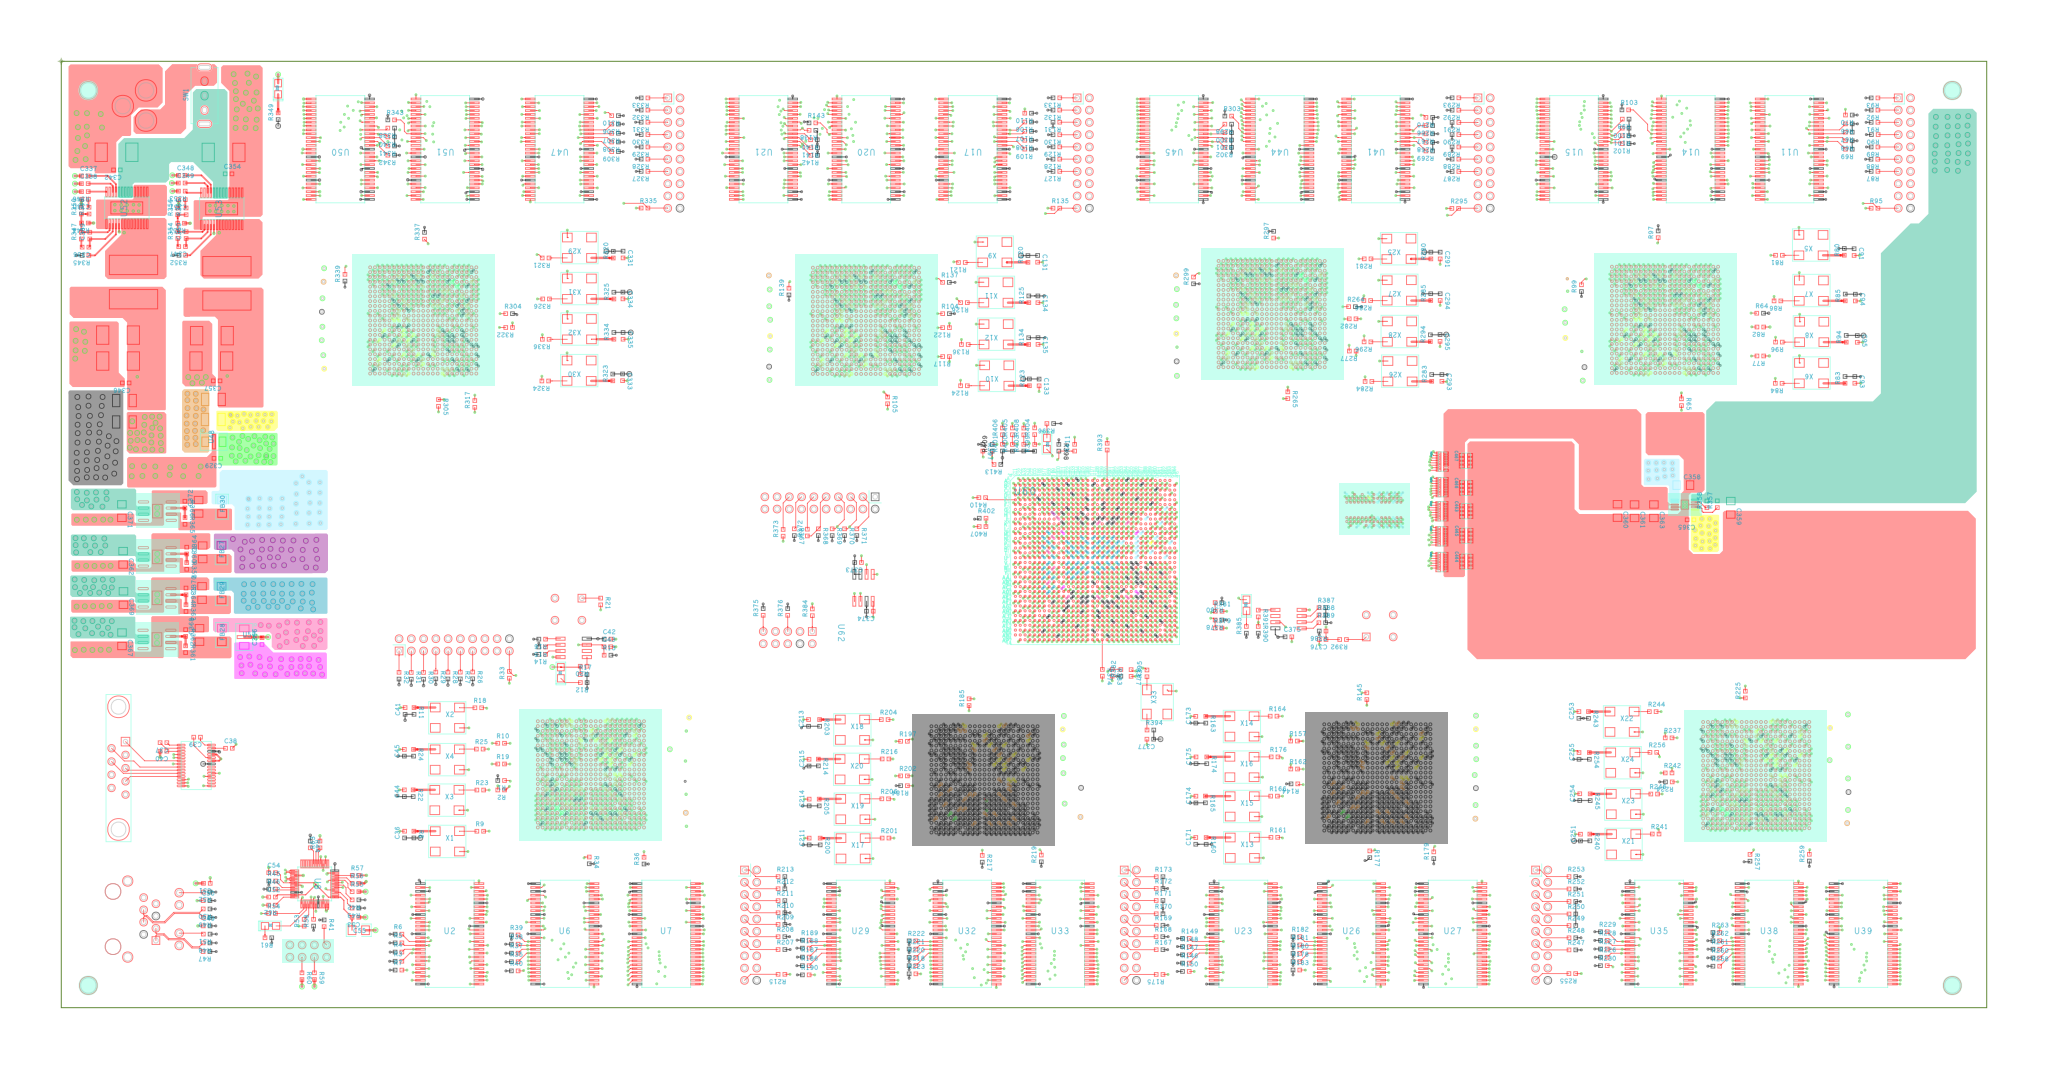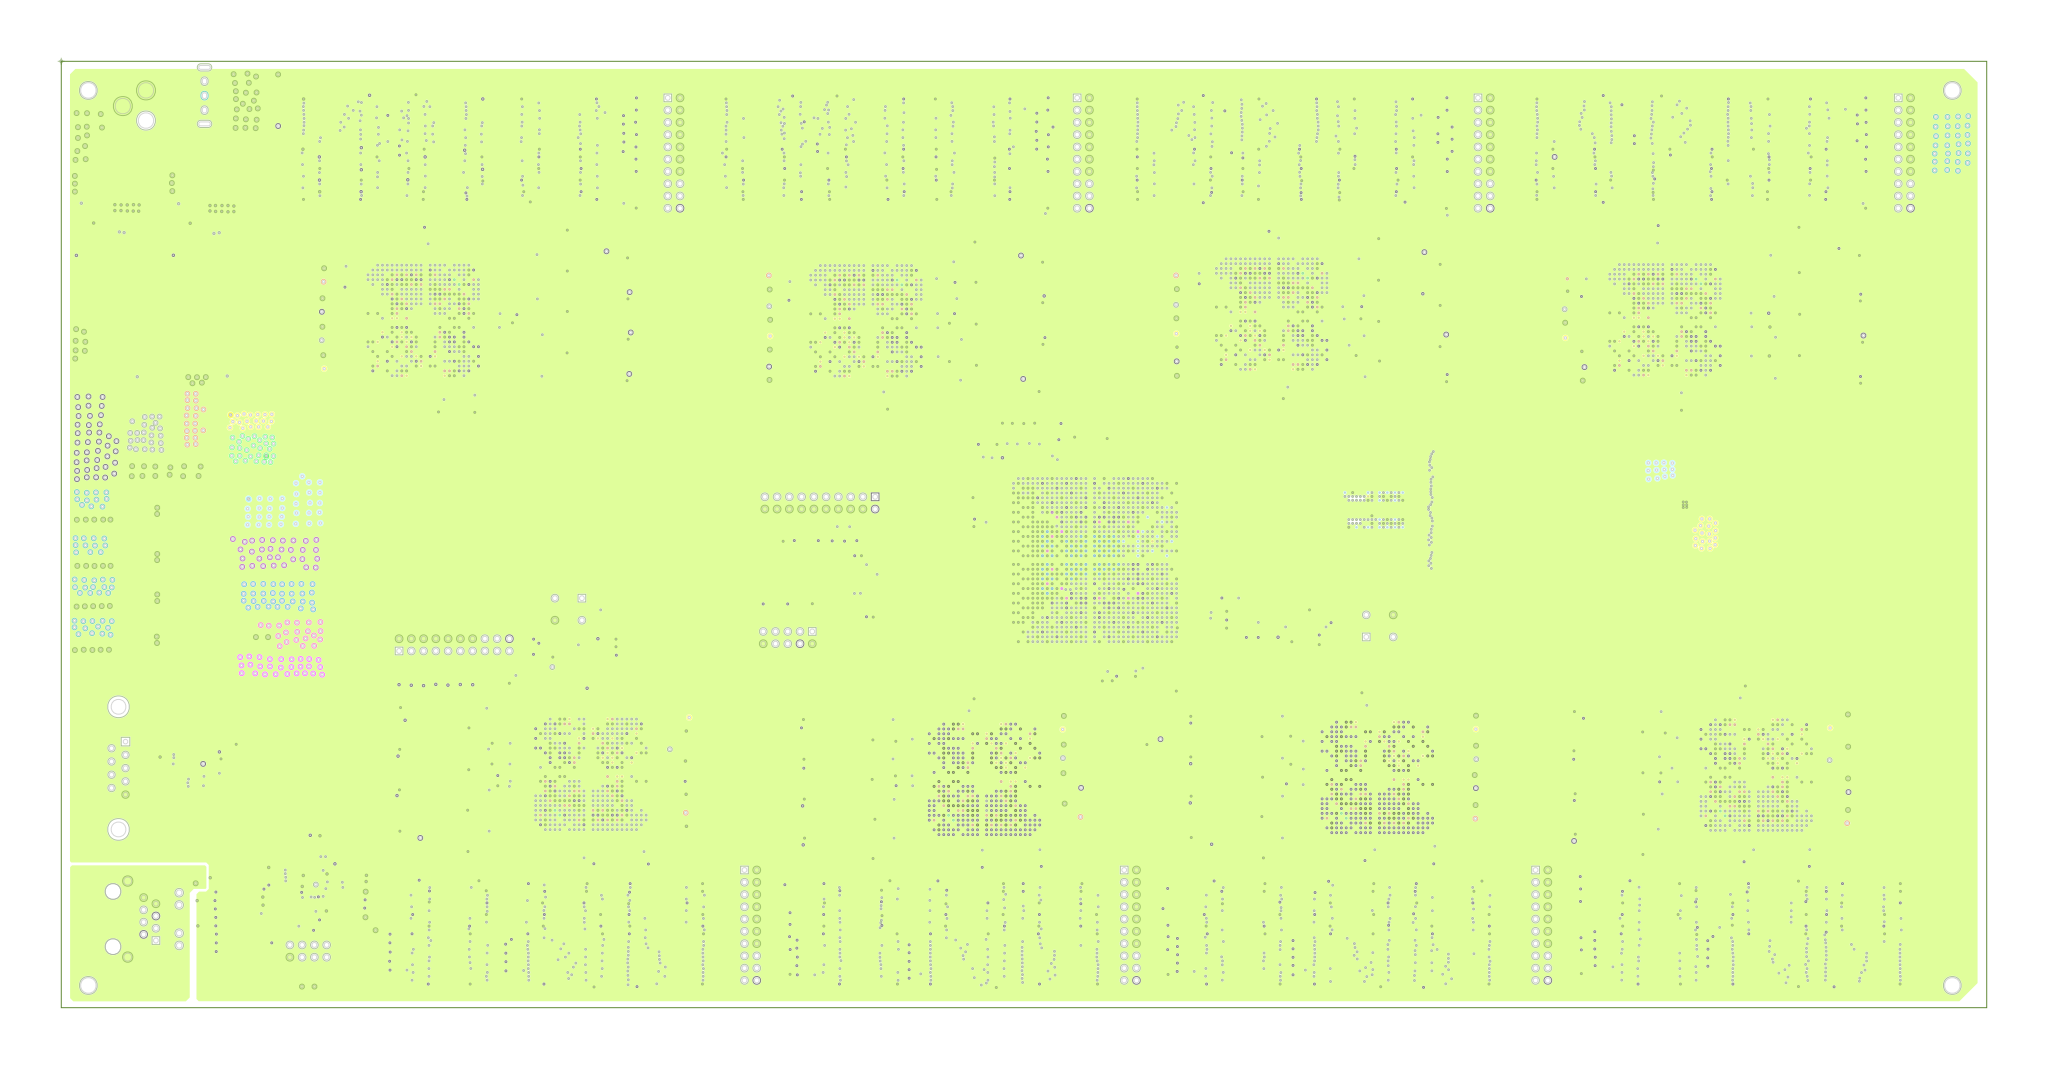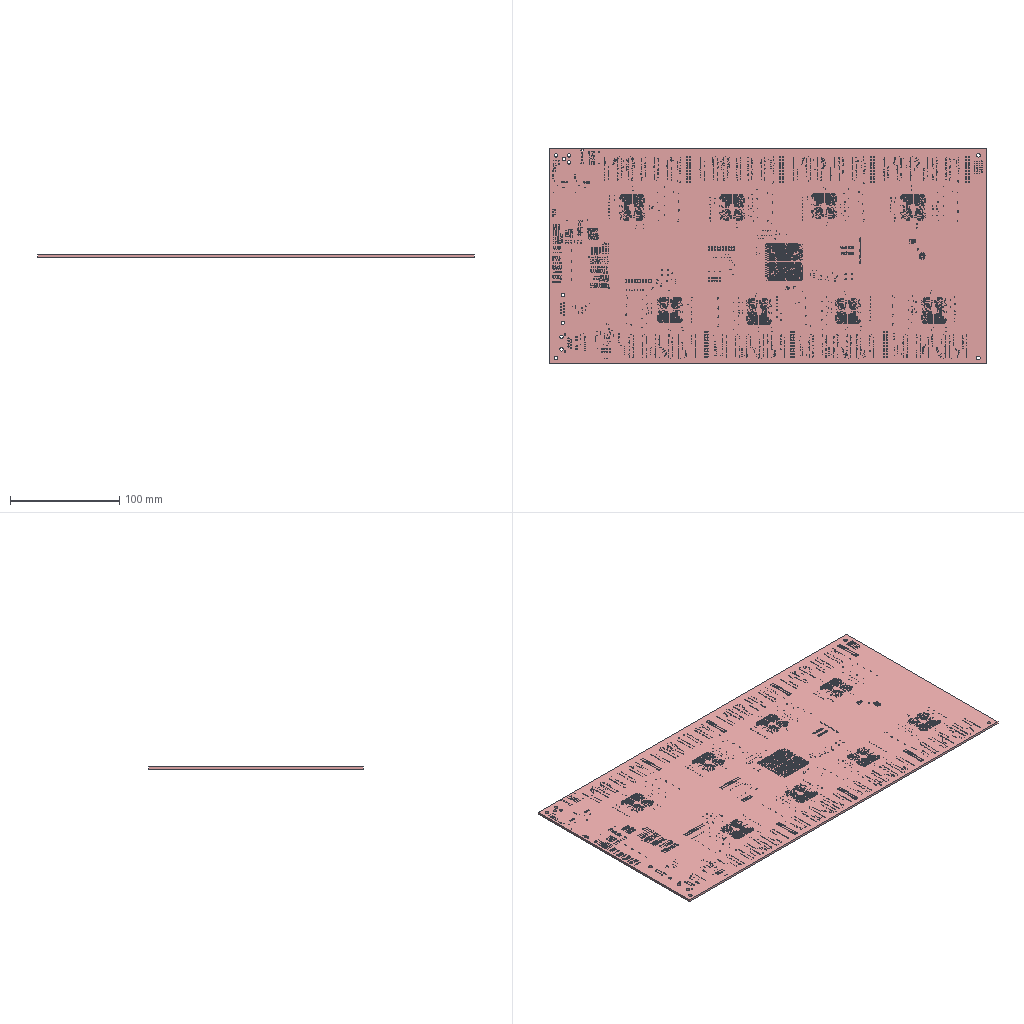Circuit board layout | Cadence Allegro | box 399 x 196 x 2.1 mm
Layer stack:
# Cadence Allegro layer stack of  (unit mm; from the constraint file cross-section; dielectric type: 0 not recorded (Allegro does not mark core vs prepreg), 3 surface material)
index,name,kind,layer,copper_thickness_mm,dielectric_type,dielectric_thickness_mm,dielectric_material,dielectric_constant
0,Top Surface,other,,,,,,
1,TOP,copper,TOP,0.0305,,,,
2,Dielectric1,dielectric,,,0,0.2032,FR-4,4.5
3,GND2,copper,GND2,0.0305,,,,
4,Dielectric2,dielectric,,,0,0.2032,FR-4,4.5
5,SIG3,copper,SIG3,0.0305,,,,
6,Dielectric3,dielectric,,,0,0.2032,FR-4,4.5
7,SIG4,copper,SIG4,0.0305,,,,
8,Dielectric4,dielectric,,,0,0.2032,FR-4,4.5
9,POWER5,copper,POWER5,0.0305,,,,
10,Dielectric5,dielectric,,,0,0.2032,FR-4,4.5
11,SIG6,copper,SIG6,0.0305,,,,
12,Dielectric6,dielectric,,,0,0.2032,FR-4,4.5
13,GND7,copper,GND7,0.0305,,,,
14,Dielectric7,dielectric,,,0,0.2032,FR-4,4.5
15,SIG8,copper,SIG8,0.0305,,,,
16,Dielectric8,dielectric,,,0,0.2032,FR-4,4.5
17,POWER9,copper,POWER9,0.0305,,,,
18,Dielectric9,dielectric,,,0,0.2032,FR-4,4.5
19,BOTTOM,copper,BOTTOM,0.0305,,,,
20,Bottom Surface,other,,,,,,
# drill layer pairs: low layer,high layer
drill_pair,TOP,BOTTOM
Part placement, first 571 of 1006 lines:
REFDES,COMP_VALUE,SYM_NAME,SYM_X,SYM_Y,SYM_ROTATE,SYM_MIRROR
C1,10uF,C3216,5033.571,-5866.500,90.000,YES
C2,0.1uF,C0402,3908.307,-6248.500,180.000,YES
C3,0.1uF,C0402,4125.307,-5754.500,0.000,YES
C4,0.1uF,C0402,4606.500,-5965.622,270.000,YES
C5,0.1uF,C0402,4302.000,-6161.000,90.000,YES
C6,0.1uF,C0402,4765.000,-5437.000,90.000,YES
C7,0.1uF,C0402,4417.984,-5762.138,315.000,YES
C8,0.1uF,C0402,4702.713,-5683.752,225.000,YES
C9,0.1uF,C0402,3913.441,-5652.004,135.000,YES
C10,0.1uF,C0402,3901.358,-5417.583,135.000,YES
C11,0.1uF,C0402,3905.429,-5551.500,180.000,YES
C12,0.1uF,C0402,4415.220,-5444.098,225.000,YES
C13,0.1uF,C0402,4646.776,-5509.992,90.000,YES
C14,0.1uF,C0402,4006.571,-5817.500,270.000,YES
C15,10uF,C3216,5032.307,-6127.500,90.000,YES
C16,0.1uF,C0402,4058.996,-5880.287,225.000,YES
C17,0.1uF,C0402,4724.693,-5514.500,90.000,YES
C18,0.1uF,C0402,4293.307,-5562.500,180.000,YES
C19,0.1uF,C0402,4105.307,-5439.500,0.000,YES
C20,0.1uF,C0402,4301.500,-5475.307,270.000,YES
C21,0.1uF,C0402,4221.264,-5740.500,90.000,YES
C22,0.1uF,C0402,4263.500,-5901.736,270.000,YES
C23,0.1uF,C0402,4475.736,-5868.500,180.000,YES
C24,0.1uF,C0402,4302.622,-6069.500,270.000,YES
C25,0.1uF,C0402,4547.343,-6157.555,135.000,YES
C26,0.1uF,C0402,4696.327,-5817.551,135.000,YES
C27,0.1uF,C0402,4809.378,-5617.500,90.000,YES
C28,10uF,C3216,5034.307,-5609.500,90.000,YES
C29,0.1uF,C0402,4120.500,-5320.693,0.000,YES
C30,0.1uF,C0402,4193.307,-5490.500,270.000,YES
C31,0.1uF,C0402,4519.736,-5795.500,0.000,YES
C32,0.1uF,C0402,4611.953,-5605.512,225.000,YES
C33,10uF,C3216,5036.500,-5350.622,90.000,YES
C34,0.1uF,C0402,7198.000,-750.000,270.000,YES
C35,104,0603,1227.000,-5668.000,90.000,YES
C36,0.1uF,0603,2801.000,-6305.000,90.000,NO
C37,104,0603,833.622,-5555.500,180.000,NO
C38,104,0603,1367.500,-5601.378,0.000,NO
C39,104,0603,1108.000,-5511.000,180.000,NO
C40,104,0603,833.622,-5625.500,180.000,NO
C41,0.1uF,0603,2805.000,-5297.000,90.000,NO
C42,0.1uF,0603,4456.693,-4711.500,0.000,NO
C43,0.1uF,0603,4454.693,-4773.500,0.000,NO
C44,0.1uF,0603,2799.000,-5968.000,90.000,NO
C45,0.1uF,0603,2799.000,-5638.000,90.000,NO
C46,0.1uF,0603,2232.500,-6606.693,270.000,YES
C47,0.1uF,0603,1906.500,-6744.693,90.000,YES
C48,0.1uF,0603,2125.500,-6870.693,0.000,YES
C49,0.1uF,0603,1186.307,-7049.693,0.000,NO
C50,0.1uF,0603,1185.307,-6843.693,0.000,NO
C51,1.5uF F/2KV,0603,1187.622,-6702.500,180.000,NO
C52,0.1uF,0603,1719.693,-6814.500,0.000,NO
C53,0.1uF,0603,2399.693,-6979.500,180.000,NO
C54,0.1uF,0603,1719.693,-6615.500,0.000,NO
C55,10uF,C1206,2427.000,-7085.122,0.000,NO
C56,0.1uF,C0402,13103.000,-1712.000,90.000,YES
C57,0.1uF,C0402,13399.307,-2088.500,0.000,YES
C58,0.1uF,C0402,13373.571,-2562.965,45.000,YES
C59,0.1uF,C0402,13115.307,-2432.500,0.000,YES
C60,0.1uF,C0402,13502.307,-1671.500,0.000,YES
C61,0.1uF,C0402,12956.500,-2047.307,0.000,YES
C62,10uF,C3216,12341.571,-2493.500,90.000,YES
C63,0.1uF,C0402,12788.500,-1950.693,90.000,YES
C64,0.1uF,C0402,13102.693,-1800.500,90.000,YES
C65,0.1uF,C0402,13437.307,-1849.500,0.000,YES
C66,0.1uF,C0402,13381.693,-2265.500,90.000,YES
C67,0.1uF,C0402,12928.693,-2126.500,0.000,YES
C68,0.1uF,C0402,13359.307,-2401.500,180.000,YES
C69,0.1uF,C0402,12989.500,-2479.350,45.000,YES
C70,10uF,C3216,12344.571,-1762.500,90.000,YES
C71,0.1uF,C0402,13454.823,-1775.740,315.000,YES
C72,0.1uF,C0402,12867.307,-2068.500,0.000,YES
C73,0.1uF,C0402,13487.500,-2096.693,90.000,YES
C74,0.1uF,C0402,13257.106,-1975.984,45.000,YES
C75,0.1uF,C0402,12750.500,-2422.693,270.000,YES
C76,0.1uF,C0402,12911.984,-2336.965,90.000,YES
C77,0.1uF,C0402,13141.307,-2345.500,270.000,YES
C78,0.1uF,C0402,12926.307,-2521.500,270.000,YES
C79,0.1uF,C0402,13179.500,-2187.264,270.000,YES
C80,0.1uF,C0402,13487.264,-1988.500,90.000,YES
C81,0.1uF,C0402,13142.264,-2260.500,90.000,YES
C82,0.1uF,C0402,12594.264,-2304.500,270.000,YES
C83,10uF,C3216,12339.571,-2021.500,90.000,YES
C84,0.1uF,C0402,13280.264,-2593.500,180.000,YES
C85,0.1uF,C0402,12860.390,-2214.346,45.000,YES
C86,0.1uF,C0402,13102.264,-2508.500,180.000,YES
C87,0.1uF,C0402,13038.500,-2213.736,180.000,YES
C88,10uF,C3216,12341.571,-2255.500,90.000,YES
C89,0.1uF,C0402,2931.000,-6813.000,90.000,YES
C90,0.1uF,C0402,13058.000,-742.000,270.000,YES
C91,0.1uF,0603,14626.736,-1555.500,270.000,NO
C92,0.1uF,C0402,13856.000,-747.000,270.000,YES
C93,0.1uF,0603,14632.736,-2597.500,270.000,NO
C94,0.1uF,0603,14636.736,-1926.500,270.000,NO
C95,0.1uF,0603,14652.736,-2263.500,270.000,NO
C96,10uF,C3216,5856.500,-2489.622,90.000,YES
C97,0.1uF,C0402,6951.736,-2367.500,0.000,YES
C98,0.1uF,C0402,6979.299,-1744.339,45.000,YES
C99,0.1uF,C0402,6839.736,-2411.500,180.000,YES
C100,0.1uF,C0402,6353.996,-1861.055,45.000,YES
C101,0.1uF,C0402,6762.500,-2173.736,180.000,YES
C102,0.1uF,C0402,6427.736,-2132.500,0.000,YES
C103,0.1uF,C0402,6853.339,-2207.189,315.000,YES
C104,0.1uF,C0402,6242.736,-2486.500,90.000,YES
C105,0.1uF,C0402,6978.500,-2491.736,270.000,YES
C106,0.1uF,C0402,6585.736,-1720.500,90.000,YES
C107,0.1uF,C0402,6268.736,-1957.500,90.000,YES
C108,0.1uF,C0402,6120.264,-2510.500,270.000,YES
C109,0.1uF,C0402,6329.264,-2136.500,0.000,YES
C110,10uF,C3216,5859.000,-1746.000,90.000,YES
C111,0.1uF,C0402,6584.429,-2469.500,90.000,YES
C112,0.1uF,C0402,6585.500,-1840.429,90.000,YES
C113,0.1uF,C0402,6387.500,-2352.571,90.000,YES
C114,0.1uF,C0402,6968.772,-2104.118,90.000,YES
C115,0.1uF,C0402,6390.898,-2058.736,225.000,YES
C116,0.1uF,C0402,6733.756,-1986.291,45.000,YES
C117,0.1uF,C0402,6623.571,-2353.500,270.000,YES
C118,0.1uF,C0402,6977.571,-1996.500,90.000,YES
C119,0.1uF,C0402,6692.858,-2525.736,315.000,YES
C120,0.1uF,C0402,6919.500,-1860.571,270.000,YES
C121,0.1uF,C0402,6073.500,-2310.571,270.000,YES
C122,0.1uF,C0402,6622.571,-2272.500,90.000,YES
C123,10uF,C3216,5852.307,-1997.500,90.000,YES
C124,0.1uF,C0402,6273.000,-2329.193,45.000,YES
C125,0.1uF,C0402,6507.571,-2193.500,270.000,YES
C126,0.1uF,C0402,6766.500,-2600.429,180.000,YES
C127,0.1uF,C0402,6467.429,-2549.500,270.000,YES
C128,10uF,C3216,5854.307,-2240.500,90.000,YES
C129,0.1uF,C0402,2035.000,-745.000,270.000,YES
C130,0.1uF,C0402,2891.000,-744.000,270.000,YES
C131,0.1uF,0603,7965.571,-1610.500,270.000,NO
C132,0.1uF,C0402,3375.000,-1011.000,270.000,YES
C133,0.1uF,0603,7977.571,-2618.500,270.000,NO
C134,0.1uF,0603,7967.571,-1940.500,270.000,NO
C135,0.1uF,0603,7968.571,-2280.500,270.000,NO
C136,0.1uF,C0402,10383.571,-6101.500,180.000,YES
C137,0.1uF,C0402,10719.571,-6239.500,270.000,YES
C138,0.1uF,C0402,10464.571,-5534.500,0.000,YES
C139,0.1uF,C0402,10422.500,-5847.429,180.000,YES
C140,0.1uF,C0402,10440.429,-5682.500,270.000,YES
C141,10uF,C3216,11466.307,-5926.500,270.000,YES
C142,0.1uF,C0402,11021.000,-5995.000,270.000,YES
C143,0.1uF,C0402,10776.571,-5504.500,270.000,YES
C144,0.1uF,C0402,10342.500,-6210.429,270.000,YES
C145,0.1uF,C0402,10895.571,-5816.500,180.000,YES
C146,0.1uF,C0402,10367.343,-5627.150,135.000,YES
C147,0.1uF,C0402,11174.571,-5442.500,90.000,YES
C148,0.1uF,C0402,10895.571,-5899.500,180.000,YES
C149,0.1uF,C0402,10542.500,-5779.307,0.000,YES
C150,10uF,C3216,11465.307,-6175.500,270.000,YES
C151,0.1uF,C0402,10719.378,-6156.500,90.000,YES
C152,0.1uF,C0402,10618.500,-5977.622,90.000,YES
C153,0.1uF,C0402,10330.500,-5961.622,270.000,YES
C154,0.1uF,C0402,10902.500,-5599.378,270.000,YES
C155,0.1uF,C0402,10717.500,-5522.622,90.000,YES
C156,0.1uF,C0402,10987.378,-5701.256,135.000,YES
C157,0.1uF,C0402,10658.500,-5783.571,90.000,YES
C158,0.1uF,C0402,10503.307,-5458.500,0.000,YES
C159,0.1uF,C0402,10600.622,-5599.500,90.000,YES
C160,0.1uF,C0402,10950.484,-6093.315,315.000,YES
C161,0.1uF,C0402,11223.500,-5642.264,90.000,YES
C162,0.1uF,C0402,10658.307,-5701.500,270.000,YES
C163,10uF,C3216,11465.307,-5690.500,270.000,YES
C164,0.1uF,C0402,10798.500,-5749.693,90.000,YES
C165,0.1uF,C0402,10834.693,-5404.500,90.000,YES
C166,0.1uF,C0402,11131.307,-5696.500,180.000,YES
C167,0.1uF,C0402,11072.307,-5523.500,90.000,YES
C168,10uF,C3216,11466.307,-5445.500,270.000,YES
C169,0.1uF,C0402,3827.000,-747.000,270.000,YES
C170,0.1uF,C0402,5493.000,-924.000,270.000,YES
C171,0.1uF,0603,9255.693,-6356.500,90.000,NO
C172,0.1uF,C0402,6804.000,-1016.000,270.000,YES
C173,0.1uF,0603,9255.693,-5368.500,90.000,NO
C174,0.1uF,0603,9256.693,-6019.500,90.000,NO
C175,0.1uF,0603,9257.693,-5699.500,90.000,NO
C176,10uF,C3216,8247.307,-5913.500,270.000,YES
C177,0.1uF,C0402,7276.307,-5540.500,0.000,YES
C178,0.1uF,C0402,7196.307,-5933.500,0.000,YES
C179,0.1uF,C0402,7687.500,-5833.307,180.000,YES
C180,0.1uF,C0402,7276.307,-5461.500,180.000,YES
C181,0.1uF,C0402,7673.307,-5910.500,180.000,YES
C182,0.1uF,C0402,7972.307,-5463.500,90.000,YES
C183,0.1uF,C0402,7515.307,-6210.500,90.000,YES
C184,0.1uF,C0402,7262.264,-5751.500,135.000,YES
C185,0.1uF,C0402,7808.307,-6150.500,90.000,YES
C186,0.1uF,C0402,7176.307,-6110.500,180.000,YES
C187,0.1uF,C0402,7122.984,-6225.720,225.000,YES
C188,0.1uF,C0402,7824.500,-6011.693,270.000,YES
C189,0.1uF,C0402,7670.307,-6170.500,0.000,YES
C190,10uF,C3216,8248.307,-6161.500,270.000,YES
C191,0.1uF,C0402,7471.307,-5625.500,90.000,YES
C192,0.1uF,C0402,7787.551,-5718.256,135.000,YES
C193,0.1uF,C0402,7514.307,-5542.500,90.000,YES
C194,0.1uF,C0402,7511.500,-6121.307,270.000,YES
C195,0.1uF,C0402,7744.350,-6109.913,45.000,YES
C196,0.1uF,C0402,7236.307,-6051.500,180.000,YES
C197,0.1uF,C0402,7110.500,-5947.307,0.000,YES
C198,0.1uF,C0402,7787.177,-5448.402,135.000,YES
C199,0.1uF,C0402,7697.500,-5624.693,270.000,YES
C200,0.1uF,C0402,7413.264,-5953.500,270.000,YES
C201,0.1uF,C0402,8019.264,-5657.500,90.000,YES
C202,0.1uF,C0402,7401.264,-5671.500,270.000,YES
C203,10uF,C3216,8246.307,-5681.500,270.000,YES
C204,0.1uF,C0402,7336.264,-5370.500,0.000,YES
C205,0.1uF,C0402,7586.224,-5761.854,45.000,YES
C206,0.1uF,C0402,7768.264,-5834.500,270.000,YES
C207,0.1uF,C0402,7866.500,-5539.622,90.000,YES
C208,10uF,C3216,8243.307,-5447.500,270.000,YES
C209,0.1uF,C0402,7676.000,-1013.000,270.000,YES
C210,0.1uF,C0402,8843.000,-749.000,270.000,YES
C211,0.1uF,0603,6101.736,-6361.500,90.000,NO
C212,0.1uF,C0402,9320.000,-1016.000,270.000,YES
C213,0.1uF,0603,6096.736,-5394.500,90.000,NO
C214,0.1uF,0603,6101.736,-6043.500,90.000,NO
C215,0.1uF,0603,6100.736,-5718.500,90.000,NO
C216,10uF,C3216,14509.307,-5958.500,270.000,YES
C217,0.1uF,C0402,13920.264,-5443.500,270.000,YES
C218,0.1uF,C0402,13887.264,-5662.500,0.000,YES
C219,0.1uF,C0402,13475.264,-6076.500,180.000,YES
C220,0.1uF,C0402,13579.264,-5439.500,180.000,YES
C221,0.1uF,C0402,13987.264,-5794.500,180.000,YES
C222,0.1uF,C0402,14117.500,-5976.736,270.000,YES
C223,0.1uF,C0402,13435.500,-6191.736,270.000,YES
C224,0.1uF,C0402,13631.500,-5759.736,0.000,YES
C225,0.1uF,C0402,13514.264,-5846.500,180.000,YES
C226,0.1uF,C0402,13809.500,-6161.264,90.000,YES
C227,0.1uF,C0402,13532.264,-5938.500,0.000,YES
C228,0.1uF,C0402,13533.264,-5660.500,270.000,YES
C229,0.1uF,C0402,14270.264,-5424.500,90.000,YES
C230,10uF,C3216,14507.307,-6213.500,270.000,YES
C231,0.1uF,C0402,14000.264,-5582.500,270.000,YES
C232,0.1uF,C0402,13655.996,-5953.874,45.000,YES
C233,0.1uF,C0402,13690.736,-5426.500,90.000,YES
C234,0.1uF,C0402,13810.500,-5464.264,270.000,YES
C235,0.1uF,C0402,14003.925,-5874.469,45.000,YES
C236,0.1uF,C0402,13731.500,-5744.736,90.000,YES
C237,0.1uF,C0402,13421.165,-5912.126,45.000,YES
C238,0.1uF,C0402,13808.689,-6094.862,0.000,YES
C239,0.1uF,C0402,13768.500,-5582.622,90.000,YES
C240,0.1uF,C0402,13869.000,-5562.000,0.000,YES
C241,0.1uF,C0402,14312.378,-5624.500,90.000,YES
C242,0.1uF,C0402,13770.500,-5665.378,270.000,YES
C243,10uF,C3216,14507.307,-5698.500,270.000,YES
C244,0.1uF,C0402,14163.500,-5504.622,90.000,YES
C245,0.1uF,C0402,14218.500,-5678.622,180.000,YES
C246,0.1uF,C0402,13628.622,-5331.500,0.000,YES
C247,0.1uF,C0402,14131.520,-5604.358,225.000,YES
C248,10uF,C3216,14506.307,-5435.500,270.000,YES
C249,0.1uF,C0402,5494.000,-747.000,270.000,YES
C250,0.1uF,C0402,2041.000,-917.000,270.000,YES
C251,0.1uF,0603,12394.500,-6329.622,90.000,NO
C252,0.1uF,C0402,2516.000,-1012.000,270.000,YES
C253,0.1uF,0603,12381.500,-5329.622,90.000,NO
C254,0.1uF,0603,12388.500,-5999.622,90.000,NO
C255,0.1uF,0603,12382.500,-5663.622,90.000,NO
C256,10uF,C3216,9166.307,-2446.500,90.000,YES
C257,0.1uF,C0402,9432.264,-2452.500,270.000,YES
C258,0.1uF,C0402,10164.571,-2517.693,45.000,YES
C259,0.1uF,C0402,10324.693,-2391.815,315.000,YES
C260,0.1uF,C0402,9716.500,-2081.622,0.000,YES
C261,0.1uF,C0402,10277.673,-1695.965,45.000,YES
C262,0.1uF,C0402,10229.500,-1803.622,0.000,YES
C263,0.1uF,C0402,10282.622,-1932.500,90.000,YES
C264,0.1uF,C0402,10160.378,-2166.500,270.000,YES
C265,0.1uF,C0402,9894.500,-2374.622,0.000,YES
C266,0.1uF,C0402,9581.500,-1904.378,90.000,YES
C267,0.1uF,C0402,9954.500,-1843.622,270.000,YES
C268,0.1uF,C0402,10071.500,-2120.378,180.000,YES
C269,0.1uF,C0402,9584.642,-2153.650,225.000,YES
C270,10uF,C3216,9164.307,-1745.500,90.000,YES
C271,0.1uF,C0402,9970.622,-2140.500,270.000,YES
C272,0.1uF,C0402,10125.307,-1802.984,135.000,YES
C273,0.1uF,C0402,10010.693,-2294.500,270.000,YES
C274,0.1uF,C0402,10046.209,-1927.815,45.000,YES
C275,0.1uF,C0402,10249.307,-2021.500,180.000,YES
C276,0.1uF,C0402,9539.307,-2374.500,270.000,YES
C277,0.1uF,C0402,10003.016,-2467.106,315.000,YES
C278,0.1uF,C0402,9704.480,-2005.571,225.000,YES
C279,0.1uF,C0402,9893.500,-1726.307,270.000,YES
C280,0.1uF,C0402,9705.500,-2293.693,90.000,YES
C281,0.1uF,C0402,9383.500,-2256.307,270.000,YES
C282,0.1uF,C0402,9622.398,-2430.965,45.000,YES
C283,10uF,C3216,9164.307,-1985.500,90.000,YES
C284,0.1uF,C0402,9894.307,-2457.500,180.000,YES
C285,0.1uF,C0402,9813.307,-2147.500,270.000,YES
C286,0.1uF,C0402,9479.307,-2199.500,0.000,YES
C287,0.1uF,C0402,9777.307,-2489.500,270.000,YES
C288,10uF,C3216,9164.307,-2220.500,90.000,YES
C289,0.1uF,C0402,3828.000,-919.000,270.000,YES
C290,0.1uF,C0402,4305.000,-829.000,270.000,YES
C291,0.1uF,0603,11249.693,-1583.500,270.000,NO
C292,0.1uF,C0402,6331.000,-917.000,270.000,YES
C293,0.1uF,0603,11263.693,-2581.500,270.000,NO
C294,0.1uF,0603,11249.693,-1922.500,270.000,NO
C295,0.1uF,0603,11248.693,-2255.500,270.000,NO
C296,10uF,C3216,2212.500,-2042.378,270.000,YES
C297,0.1uF,C0402,2508.693,-2505.500,270.000,YES
C298,0.1uF,C0402,3287.693,-1837.500,0.000,YES
C299,0.1uF,C0402,3200.500,-2486.693,45.000,YES
C300,0.1uF,C0402,2733.693,-2132.500,0.000,YES
C301,0.1uF,C0402,2659.500,-1970.307,90.000,YES
C302,0.1uF,C0402,2696.693,-1836.500,180.000,YES
C303,0.1uF,C0402,3326.693,-1719.500,0.000,YES
C304,0.1uF,C0402,3270.551,-2089.598,0.000,YES
C305,0.1uF,C0402,3417.622,-2450.945,315.000,YES
C306,0.1uF,C0402,3070.693,-1936.500,90.000,YES
C307,0.1uF,C0402,2970.693,-1850.500,90.000,YES
C308,0.1uF,C0402,3149.693,-2169.500,180.000,YES
C309,0.1uF,C0402,3295.669,-2171.965,315.000,YES
C310,10uF,C3216,2209.500,-1797.378,270.000,YES
C311,0.1uF,C0402,2617.673,-2525.906,135.000,YES
C312,0.1uF,C0402,2704.469,-2252.417,315.000,YES
C313,0.1uF,C0402,3128.610,-1974.945,45.000,YES
C314,0.1uF,C0402,2922.500,-2362.736,180.000,YES
C315,0.1uF,C0402,2784.075,-2060.217,315.000,YES
C316,0.1uF,C0402,3059.264,-2186.500,270.000,YES
C317,0.1uF,C0402,2735.736,-1758.500,0.000,YES
C318,0.1uF,C0402,3011.736,-1758.500,0.000,YES
C319,0.1uF,C0402,3248.736,-1916.500,0.000,YES
C320,0.1uF,C0402,3009.736,-2329.500,270.000,YES
C321,0.1uF,C0402,3009.736,-2244.500,90.000,YES
C322,0.1uF,C0402,2464.500,-2307.736,270.000,YES
C323,10uF,C3216,2217.500,-2274.378,270.000,YES
C324,0.1uF,C0402,3147.500,-2598.264,180.000,YES
C325,0.1uF,C0402,2972.736,-2466.500,180.000,YES
C326,0.1uF,C0402,2578.736,-2270.500,0.000,YES
C327,0.1uF,C0402,2545.736,-2430.500,270.000,YES
C328,10uF,C3216,2218.500,-2506.378,270.000,YES
C329,0.1uF,0603,1273.500,-3237.264,180.000,NO
C330,0.1uF,C0402,6330.000,-748.000,270.000,YES
C331,0.1uF,0603,4583.264,-1575.500,270.000,NO
C332,0.1uF,C0402,7200.000,-918.000,270.000,YES
C333,0.1uF,0603,4579.264,-2576.500,270.000,NO
C334,0.1uF,0603,4582.264,-1909.500,270.000,NO
C335,0.1uF,0603,4583.264,-2238.500,270.000,NO
C336,120p,0603,197.500,-1515.264,180.000,NO
C337,0.1uF,0603,191.736,-934.500,0.000,NO
C338,0.039uF,0603,191.736,-997.500,0.000,NO
C339,5600p,0603,232.500,-1421.264,90.000,NO
C340,8200p,0603,194.500,-1124.264,180.000,NO
C341,0.047uF,0603,488.000,-1347.000,180.000,YES
C342,0.1uF,0603,453.736,-885.500,180.000,NO
C343,470uF,C7343,575.736,-741.500,180.000,NO
C344,470uF,C7343,588.000,-2444.000,180.000,NO
C345,470uF,C7343,587.736,-2232.500,180.000,NO
C346,100p,0603,525.736,-2622.500,180.000,NO
C347,120p,0603,985.736,-1510.500,180.000,NO
C348,0.1uF,0603,982.736,-929.500,0.000,NO
C349,0.039uF,0603,982.736,-992.500,0.000,NO
C350,5600p,0603,1018.500,-1417.264,90.000,NO
C351,8200p,0603,984.500,-1127.736,180.000,NO
C352,0.047uF,0603,1262.000,-1357.000,180.000,YES
C353,470uF,C7343,1199.000,-743.000,0.000,NO
C354,0.1uF,0603,1364.736,-917.500,0.000,NO
C355,470uF,C7343,1354.000,-2237.000,180.000,NO
C356,470uF,C7343,1349.000,-2444.000,180.000,NO
C357,100p,0603,1267.500,-2605.378,180.000,NO
C358,10uF,C3216,13178.500,-3455.622,0.000,NO
C359,10uF,C3216,13620.622,-3585.500,270.000,NO
C360,10uF,C3216,12696.500,-3611.378,270.000,NO
C361,10uF,C3216,12835.500,-3613.378,270.000,NO
C362,10uF,C3216,504.500,-3993.622,270.000,NO
C363,10uF,C3216,12993.500,-3613.378,270.000,NO
C364,10uF,C3216,1153.622,-4058.500,90.000,NO
C365,0.1uF,0603,13292.264,-3738.500,180.000,NO
C366,0.1uF,0603,1637.500,-4727.264,90.000,NO
C367,10uF,C3216,495.378,-4657.500,270.000,NO
C368,10uF,C3216,1127.500,-4732.571,90.000,NO
C369,10uF,C3216,507.429,-4321.500,270.000,NO
C370,10uF,C3216,1148.429,-4390.500,90.000,NO
C371,10uF,C3216,494.500,-3612.429,270.000,NO
C372,10uF,C3216,1120.500,-3687.571,90.000,NO
C373,0.1uF,0603,6500.736,-4086.500,180.000,NO
C374,0.1uF,0603,6596.736,-4483.500,180.000,NO
C375,0.1uF,0603,10011.736,-4692.500,0.000,NO
C376,0.1uF,0603,10290.736,-4714.500,180.000,NO
C377,0.1uF,0603,8884.500,-5527.264,180.000,NO
C378,0.1uF,C0402,8883.209,-3913.087,0.000,YES
C379,0.1uF,C0402,8115.654,-4109.913,225.000,YES
C380,0.1uF,C0402,8111.307,-3761.185,45.000,YES
C381,0.1uF,C0402,8117.571,-3909.307,135.000,YES
C382,0.1uF,C0402,8508.016,-3755.693,135.000,YES
C383,0.1uF,C0402,8669.500,-4342.622,315.000,YES
C384,0.1uF,C0402,8488.500,-4377.622,270.000,YES
C385,0.1uF,C0402,2520.000,-819.000,270.000,YES
C386,0.1uF,C0402,8044.693,-4240.500,270.000,YES
C387,0.1uF,C0402,8705.500,-3774.622,90.000,YES
C388,0.1uF,C0402,8006.520,-4010.429,0.000,YES
C389,0.1uF,C0402,8059.500,-3716.622,0.000,YES
C390,0.1uF,C0402,8567.693,-4456.500,90.000,YES
C391,0.1uF,C0402,9050.500,-4387.622,90.000,YES
C392,0.1uF,C0402,8965.378,-4618.500,90.000,YES
C393,0.1uF,C0402,8396.500,-4439.622,90.000,YES
C394,0.1uF,C0402,8254.622,-4414.500,90.000,YES
C395,0.1uF,C0402,7967.965,-3519.957,315.000,YES
C396,0.1uF,C0402,8375.000,-3751.000,90.000,YES
C397,0.1uF,C0402,8241.500,-3697.622,0.000,YES
C398,0.1uF,C0402,8665.000,-3698.000,180.000,YES
C399,0.1uF,C0402,8395.500,-3620.622,180.000,YES
C400,0.1uF,C0402,8818.500,-4294.622,135.000,YES
C401,0.1uF,C0402,8160.236,-4496.531,45.000,YES
C402,0.1uF,C0402,8471.402,-3675.280,225.000,YES
C403,0.1uF,C0402,8744.622,-4337.500,315.000,YES
C404,0.1uF,C0402,8511.307,-3497.843,0.000,YES
C405,0.1uF,C0402,8464.965,-3407.087,225.000,YES
C406,0.1uF,C0402,8929.500,-4070.622,180.000,YES
C407,0.1uF,C0402,8547.791,-4379.740,225.000,YES
C408,0.1uF,C0402,8040.720,-4414.331,315.000,YES
C409,0.1uF,C0402,8031.378,-4490.500,270.000,YES
C410,0.1uF,C0402,8433.693,-4008.500,0.000,YES
C411,0.1uF,C0402,8512.500,-4126.941,180.000,YES
C412,0.1uF,C0402,8237.500,-3928.941,180.000,YES
C413,0.1uF,C0402,8395.059,-4159.500,90.000,YES
C414,0.1uF,C0402,8124.102,-3990.535,135.000,YES
C415,0.1uF,C0402,8393.500,-4072.941,180.000,YES
C416,0.1uF,C0402,8604.500,-4066.941,0.000,YES
C417,0.1uF,C0402,8080.720,-4066.335,0.000,YES
C418,0.1uF,C0402,7995.500,-4064.941,0.000,YES
C419,0.1uF,C0402,7994.091,-4309.969,45.000,YES
C420,0.1uF,C0402,8276.500,-4007.941,0.000,YES
C421,0.1uF,C0402,8189.091,-4194.969,45.000,YES
C422,0.1uF,C0402,8197.500,-4086.941,0.000,YES
C423,0.1uF,C0402,8591.500,-4007.941,0.000,YES
C424,0.1uF,C0402,7993.346,-3862.949,315.000,YES
C425,0.1uF,C0402,8512.500,-4058.941,180.000,YES
C426,0.1uF,C0402,8394.941,-3943.500,270.000,YES
C427,0.1uF,C0402,8122.748,-4262.283,225.000,YES
C428,0.1uF,C0402,8281.500,-4064.941,180.000,YES
C429,0.1uF,C0402,8394.902,-3857.571,270.000,YES
C430,0.1uF,C0402,8210.004,-4346.673,315.000,YES
C431,0.1uF,C0402,2893.000,-921.000,270.000,YES
C432,0.1uF,C0402,3375.000,-828.000,270.000,YES
C433,0.1uF,C0402,4303.000,-1016.000,270.000,YES
C434,0.1uF,C0402,5968.000,-1015.000,270.000,YES
C435,0.1uF,C0402,5969.000,-825.000,270.000,YES
C436,0.1uF,C0402,6805.000,-823.000,270.000,YES
C437,0.1uF,C0402,7677.000,-824.000,270.000,YES
C438,0.1uF,C0402,8843.000,-921.000,270.000,YES
C439,0.1uF,C0402,10489.000,-919.000,270.000,YES
C440,0.1uF,C0402,10640.000,-3449.941,270.000,YES
C441,0.1uF,C0402,10962.000,-825.000,270.000,YES
C442,0.1uF,C0402,13056.000,-922.000,270.000,YES
C443,0.1uF,C0402,13271.000,-7082.000,90.000,YES
C444,0.1uF,C0402,11589.000,-7083.000,90.000,YES
C445,0.1uF,C0402,9879.000,-7082.000,90.000,YES
C446,0.1uF,C0402,9407.000,-6997.000,90.000,YES
C447,0.1uF,C0402,10809.500,-3449.941,270.000,YES
C448,0.1uF,C0402,10749.500,-3449.941,270.000,YES
C449,0.1uF,C0402,10697.500,-3449.941,270.000,YES
C450,0.1uF,C0402,10869.500,-3449.941,270.000,YES
C451,0.1uF,C0402,10740.500,-3864.941,90.000,YES
C452,0.1uF,C0402,10681.500,-3864.941,90.000,YES
C453,0.1uF,C0402,10930.500,-3864.941,90.000,YES
C454,0.1uF,C0402,7908.000,-6812.000,90.000,YES
C455,0.1uF,C0402,10800.000,-3864.941,90.000,YES
C456,0.1uF,C0402,10863.500,-3864.941,90.000,YES
C457,0.1uF,C0402,10586.500,-3864.941,90.000,YES
C458,0.1uF,C0402,10487.500,-3449.941,270.000,YES
C459,0.1uF,C0402,4343.000,-7083.000,90.000,YES
C460,0.1uF,C0402,10716.500,-3660.941,0.000,YES
C461,0.1uF,C0402,10886.500,-3662.941,180.000,YES
C462,0.1uF,C0402,10937.500,-3449.941,270.000,YES
C463,CP,CA-AVE-0603-8,11462.000,-3668.000,270.000,NO
C464,CP,CA-AVE-0603-8,11463.000,-4079.000,270.000,NO
C465,CP,CA-AVE-0603-8,11463.000,-3868.000,270.000,NO
C466,CP,CA-AVE-0603-8,11461.000,-3478.000,270.000,NO
C467,CP,CA-AVE-0603-8,11460.000,-3257.000,270.000,NO
C468,0.1uF,C0402,9702.000,-746.000,270.000,YES
C469,0.1uF,C0402,10486.000,-747.000,270.000,YES
C470,0.1uF,C0402,12106.000,-918.000,270.000,YES
C471,0.1uF,C0402,14176.000,-7081.000,90.000,YES
C472,0.1uF,C0402,12799.000,-7003.000,90.000,YES
C473,0.1uF,C0402,11588.000,-6905.000,90.000,YES
C474,0.1uF,C0402,9879.000,-6909.000,90.000,YES
C475,0.1uF,C0402,6762.000,-7083.000,90.000,YES
C476,0.1uF,C0402,6285.000,-6809.000,90.000,YES
C477,0.1uF,C0402,4699.000,-7000.000,90.000,YES
C478,0.1uF,C0402,10181.000,-1012.000,270.000,YES
C479,0.1uF,C0402,10178.000,-824.000,270.000,YES
C480,0.1uF,C0402,12103.000,-750.000,270.000,YES
C481,0.1uF,C0402,14173.000,-6907.000,90.000,YES
C482,0.1uF,C0402,11115.000,-6812.000,90.000,YES
C483,0.1uF,C0402,11114.000,-7003.000,90.000,YES
C484,0.1uF,C0402,9405.000,-6814.000,90.000,YES
C485,0.1uF,C0402,7909.000,-7002.000,90.000,YES
C486,0.1uF,C0402,7629.000,-7077.000,90.000,YES
C487,0.1uF,C0402,7155.000,-7002.000,90.000,YES
C488,0.1uF,C0402,4342.000,-6909.000,90.000,YES
C489,0.1uF,C0402,3871.000,-7002.000,90.000,YES
C490,0.1uF,C0402,12580.000,-822.000,270.000,YES
C491,0.1uF,C0402,13533.000,-1013.000,270.000,YES
C492,0.1uF,C0402,14341.000,-1015.000,270.000,YES
C493,0.1uF,C0402,14339.000,-827.000,270.000,YES
C494,0.1uF,C0402,9320.000,-811.000,270.000,YES
C495,0.1uF,C0402,9704.000,-917.000,270.000,YES
C496,0.1uF,C0402,10964.000,-1009.000,270.000,YES
C497,0.1uF,C0402,13698.000,-6814.000,90.000,YES
C498,0.1uF,C0402,13695.000,-6999.000,90.000,YES
C499,0.1uF,C0402,13274.000,-6908.000,90.000,YES
C500,0.1uF,C0402,12800.000,-6815.000,90.000,YES
C501,0.1uF,C0402,5172.000,-7081.000,90.000,YES
C502,0.1uF,C0402,6759.000,-6910.000,90.000,YES
C503,0.1uF,C0402,5170.000,-6906.000,90.000,YES
C504,0.1uF,C0402,4697.000,-6812.000,90.000,YES
C505,0.1uF,C0402,3406.000,-6909.000,90.000,YES
C506,0.1uF,C0402,12580.000,-1014.000,270.000,YES
C507,0.1uF,C0402,13862.000,-922.000,270.000,YES
C508,0.1uF,C0402,14462.000,-7007.000,90.000,YES
C509,0.1uF,C0402,14944.000,-6910.000,90.000,YES
C510,0.1uF,C0402,3405.000,-7086.000,90.000,YES
C511,0.1uF,C0402,13532.000,-827.000,270.000,YES
C512,0.1uF,C0402,14465.000,-6817.000,90.000,YES
C513,0.1uF,C0402,14942.000,-7083.000,90.000,YES
C514,0.1uF,C0402,10766.000,-6908.000,90.000,YES
C515,0.1uF,C0402,8384.000,-7082.000,90.000,YES
C516,0.1uF,C0402,8390.000,-6912.000,90.000,YES
C517,0.1uF,C0402,7629.000,-6909.000,90.000,YES
C518,0.1uF,C0402,10763.000,-7080.000,90.000,YES
C519,0.1uF,C0402,10286.000,-7004.000,90.000,YES
C520,0.1uF,C0402,10286.000,-6814.000,90.000,YES
C521,0.1uF,C0402,7152.000,-6815.000,90.000,YES
C522,0.1uF,C0402,6284.000,-7002.000,90.000,YES
C523,0.1uF,C0402,3868.000,-6818.000,90.000,YES
C524,0.1uF,C0402,2929.000,-7000.000,90.000,YES
D1,LED RED,LED0805,4075.681,-4985.551,90.000,NO
D2,LED YELLOW,LED0805,1707.000,-7050.000,0.000,NO
D10,LED YELLOW,LED0805,1769.000,-224.000,90.000,NO
D11,LED RED,LED0805,9669.551,-4434.957,90.000,NO
D12,LED,LED0805,8041.138,-3116.512,270.000,NO
FB22,BLM21PG331SN1-0805,1210,510.512,-2933.736,0.000,NO
FB23,BLM21PG331SN1-0805,1210,1235.488,-2913.406,0.000,NO
FB25,BLM21PG331SN1-1206,1210,519.807,-2773.110,180.000,NO
FB26,BLM21PG331SN1-1206,1210,1245.764,-2764.000,180.000,NO
FB27,BLM21PG331SN1-1206,C1206,1307.000,-4002.764,90.000,NO
FB28,BLM21PG331SN1-1206,C1206,1310.000,-4677.764,90.000,NO
FB29,BLM21PG331SN1-1206,C1206,1308.000,-4335.764,90.000,NO
FB30,BLM21PG331SN1-1206,C1206,1312.000,-3631.764,90.000,NO
J1,JTAG_HEADER_2X10,JTAG_HEADER_2X10,2756.000,-4808.000,90.000,NO
J2,JTAG_HEADER_2X10,JTAG_HEADER_2X10,14987.000,-298.000,0.000,NO
J3,JTAG_HEADER_2X10,JTAG_HEADER_2X10,8287.882,-298.000,0.000,NO
J4,JTAG_HEADER_2X10,JTAG_HEADER_2X10,8672.000,-6594.000,0.000,NO
J5,JTAG_HEADER_2X10,JTAG_HEADER_2X10,5574.000,-6594.000,0.000,NO
J6,JTAG_HEADER_2X10,JTAG_HEADER_2X10,12028.000,-6594.000,0.000,NO
J7,JTAG_HEADER_2X10,JTAG_HEADER_2X10,11558.000,-298.000,0.000,NO
J8,JTAG_HEADER_2X10,JTAG_HEADER_2X10,4948.000,-298.000,0.000,NO
J9,CON3,CON_POWER,691.122,-483.000,90.000,NO
J10,JTAG_HEADER_2X10,JTAG_HEADER_2X10,6640.000,-3550.882,270.000,NO
JP1,DB9,DB9-MALE,462.980,-6263.173,270.000,NO
JP2,RJ45_J1012F21KNL,RJ45_J1012F21KNL,672.000,-6819.000,270.000,NO
L1,4.7uH,INC5A,589.287,-1660.161,270.000,NO
L2,4.7uH,INC5A,1351.287,-1670.484,270.000,NO
R1,10K,0603,3588.571,-5864.000,180.000,NO
R2,0,0603,3588.571,-5941.500,180.000,NO
R3,10K,0603,2751.000,-7338.000,0.000,NO
R4,10K,0603,2751.000,-7263.000,0.000,NO
R5,10K,0603,2751.000,-7188.000,0.000,NO
R6,10K,0603,2751.000,-7117.000,0.000,NO
R7,10K,0603,2751.000,-7410.000,0.000,NO
R8,33,0603,2877.000,-6305.000,270.000,NO
R9,33,0603,3418.000,-6278.000,0.000,NO
R10,23.6K 1%,0603,3588.571,-5560.500,0.000,NO
R11,33,0603,2878.000,-5297.000,270.000,NO
R12,360,0603,4262.429,-5065.500,180.000,NO
R13,10K,0603,4456.693,-4842.500,0.000,NO
R14,10K,0603,3923.429,-4835.500,180.000,NO
R15,10K,0603,3923.500,-4775.622,180.000,NO
R16,10K,0603,3923.500,-4711.622,180.000,NO
R17,1K,0603,4261.429,-5000.500,0.000,NO
R18,33,0603,3402.000,-5271.000,0.000,NO
R19,12.1K 1%,0603,3588.571,-5729.500,0.000,NO
Pad and via stacks:
# Allegro (Cadence) via spans and padstacks; design units: ("mils" 3 1000)
# via spans: padstack,start_layer,end_layer,net_example,count
VIA8_16,ETCH/TOP,ETCH/BOTTOM,UA_RXD0_232_J,5584
VIA20C10D,ETCH/TOP,ETCH/BOTTOM,VCC3P3V,95
VIA20D40,ETCH/TOP,ETCH/BOTTOM,GND,545
# Allegro padstack definitions: name,start_layer,end_layer,drill,plating,holeType,type
SMD3216,"ETCH/TOP","ETCH/TOP",0.0,"PLATED","none","smd"
SMD0603,"ETCH/TOP","ETCH/TOP",0.0,"PLATED","none","smd"
SMD7343,"ETCH/TOP","ETCH/TOP",0.0,"PLATED","none","smd"
SMD1R60X1R80,"ETCH/TOP","ETCH/TOP",0.0,"PLATED","none","smd"
R1N50X1N40,"ETCH/TOP","ETCH/TOP",0.0,"PLATED","none","smd"
R4_0X1_0,"ETCH/TOP","ETCH/TOP",0.0,"PLATED","none","smd"
SMD20X3-5,"ETCH/TOP","ETCH/TOP",0.0,"PLATED","none","smd"
SMD1_4REC1_95,"ETCH/TOP","ETCH/TOP",0.0,"PLATED","none","smd"
SMD0_6REC2_95,"ETCH/TOP","ETCH/TOP",0.0,"PLATED","none","smd"
SMD75X25,"ETCH/TOP","ETCH/TOP",0.0,"PLATED","none","smd"
OBLONG65X14,"ETCH/TOP","ETCH/TOP",0.0,"PLATED","none","smd"
R80X12,"ETCH/TOP","ETCH/TOP",0.0,"NON_PLATED","none","smd"
TPS54610_PWRPAD,"ETCH/TOP","ETCH/TOP",0.0,"PLATED","none","smd"
R61X74,"ETCH/TOP","ETCH/TOP",0.0,"PLATED","none","smd"
T10X61,"ETCH/TOP","ETCH/TOP",0.0,"PLATED","none","smd"
T78X110,"ETCH/TOP","ETCH/TOP",0.0,"PLATED","none","smd"
T17X84,"ETCH/TOP","ETCH/TOP",0.0,"PLATED","none","smd"
80X24,"ETCH/TOP","ETCH/TOP",0.0,"PLATED","none","smd"
C24,"ETCH/TOP","ETCH/TOP",0.0,"PLATED","none","smd"
SMD_1P3REC0P2,"ETCH/TOP","ETCH/TOP",0.0,"PLATED","none","smd"
SMD2_0REC1_8,"ETCH/TOP","ETCH/TOP",0.0,"PLATED","none","smd"
018RD,"ETCH/TOP","ETCH/TOP",0.0,"PLATED","none","smd"
Y23X23,"ETCH/TOP","ETCH/TOP",0.0,"PLATED","none","smd"
R30X25,"ETCH/TOP","ETCH/TOP",0.0,"PLATED","none","smd"
O24X28,"ETCH/TOP","ETCH/TOP",0.0,"PLATED","none","smd"
60X100,"ETCH/TOP","ETCH/TOP",0.0,"PLATED","none","smd"
THS1_6D1_0,"ETCH/TOP","ETCH/BOTTOM",39.37,"PLATED","circle_drill","through"
THC1_6D1_0,"ETCH/TOP","ETCH/BOTTOM",39.37,"PLATED","circle_drill","through"
PAD10,"ETCH/TOP","ETCH/BOTTOM",125.0,"PLATED","circle_drill","through"
PAD12,"ETCH/TOP","ETCH/BOTTOM",37.0,"PLATED","circle_drill","through"
PAD11,"ETCH/TOP","ETCH/BOTTOM",37.0,"PLATED","circle_drill","through"
PAD13,"ETCH/TOP","ETCH/BOTTOM",120.0,"PLATED","circle_drill","through"
THC1_75D1_15,"ETCH/TOP","ETCH/BOTTOM",45.0,"PLATED","circle_drill","through"
H3_2_NEW,"ETCH/TOP","ETCH/BOTTOM",128.0,"NON_PLATED","circle_drill","through"
THC84D64,"ETCH/TOP","ETCH/BOTTOM",64.0,"PLATED","circle_drill","through"
THR0P8X2P4,"ETCH/TOP","ETCH/BOTTOM",31.5,"PLATED","oval slot","through"
THR0P9X1P2,"ETCH/TOP","ETCH/BOTTOM",35.429,"PLATED","oval slot","through"
DWK,"ETCH/TOP","ETCH/BOTTOM",125.984,"PLATED","circle_drill","through"
VIA8_16,"ETCH/TOP","ETCH/BOTTOM",8.0,"PLATED","circle_drill","through"
VIA20C10D,"ETCH/TOP","ETCH/BOTTOM",10.0,"PLATED","circle_drill","through"
VIA20D40,"ETCH/TOP","ETCH/BOTTOM",20.0,"PLATED","circle_drill","through"
SMD-R0-6X1-05_MM,"ETCH/TOP","ETCH/TOP",0.0,"PLATED","none","smd"
SMD-R0-3X1_MM,"ETCH/TOP","ETCH/TOP",0.0,"PLATED","none","smd"
SMD-R0-4X1_MM,"ETCH/TOP","ETCH/TOP",0.0,"PLATED","none","smd"
Design rules, without the lines most boards share, first 14 of 67 lines:
# Cadence Allegro design rules of  (from the Constraint Manager export constraints.dcfx, design unit mil; typed fields in mm)
# columns: name | kind | enabled | priority | scope1 | scope2 | descriptor | typed fields (field=value)
# Allegro precedence (priority 1 wins): 1 Region class-to-class, 2 Region class, 3 Region, 4 class-to-class, 5 DiffPair/Bus/NetGroup override, 6 NetClass, 7 constraint set (CSet) default
# per-layer values are written LAYER=value in the descriptor and LAYER:mm in the typed field; a maximum of 0 means no limit set
# --- net classes (and buses / net groups) ---
EMB7-D | NetClass | enabled | 6 | EMB7_D0, EMB7_D1, EMB7_D2, EMB7_D3, EMB7_D4, EMB7_D5, EMB7_D6, EMB7_D7, EMB7_D8, EMB7_D9, EMB7_D10, EMB7_D11, EMB7_D12, EMB7_D13, EMB7_D14, EMB7_D15, EMB7_WE_DQM0, EMB7_WE_DQM1 | All | Net Class (members: 18 Net) |
EMB7-A | NetClass | enabled | 6 | EMB7_AOE_N, EMB7_AWE_N, EMB7_A1, EMB7_A2, EMB7_A3, EMB7_A4, EMB7_A5, EMB7_A6, EMB7_A7, EMB7_A8, EMB7_A9, EMB7_A10, EMB7_A11, EMB7_A12, EMB7_A13, EMB7_BA_V2_0, EMB7_BA_V2_1, EMB7_CAS_N, EMB7_CLK, EMB7_CS0_N, EMB7_SDCKE | All | Net Class (members: 21 Net) |
EMA7-D | NetClass | enabled | 6 | EMA7_D0, EMA7_D1, EMA7_D2, EMA7_D3, EMA7_D4, EMA7_D5, EMA7_D6, EMA7_D7, EMA7_D8, EMA7_D9, EMA7_D10, EMA7_D11, EMA7_D12, EMA7_D13, EMA7_D14, EMA7_D15, EMA7_D16, EMA7_D17, EMA7_D18, EMA7_D19, EMA7_D20, EMA7_D21, EMA7_D22, EMA7_D23, EMA7_D24, EMA7_D25, EMA7_D26, EMA7_D27, EMA7_D28, EMA7_D29, EMA7_D30, EMA7_D31, EMA7_WE_DQM0, EMA7_WE_DQM1, EMA7_WE_DQM2, EMA7_WE_DQM3 | All | Net Class (members: 36 Net) |
EMA7-A | NetClass | enabled | 6 | EMA7_AOE_N, EMA7_AWE_N, EMA7_A1, EMA7_A2, EMA7_A3, EMA7_A4, EMA7_A5, EMA7_A6, EMA7_A7, EMA7_A8, EMA7_A9, EMA7_A10, EMA7_A11, EMA7_A12, EMA7_A13, EMA7_BA_V2_0, EMA7_BA_V2_1, EMA7_CAS_N, EMA7_CLK, EMA7_CS0_N, EMA7_SDCKE | All | Net Class (members: 21 Net) |
EMB6-D | NetClass | enabled | 6 | EMB6_D0, EMB6_D1, EMB6_D2, EMB6_D3, EMB6_D4, EMB6_D5, EMB6_D6, EMB6_D7, EMB6_D8, EMB6_D9, EMB6_D10, EMB6_D11, EMB6_D12, EMB6_D13, EMB6_D14, EMB6_D15, EMB6_WE_DQM0, EMB6_WE_DQM1 | All | Net Class (members: 18 Net) |
EMB6-A | NetClass | enabled | 6 | EMB6_AOE_N, EMB6_AWE_N, EMB6_A1, EMB6_A2, EMB6_A3, EMB6_A4, EMB6_A5, EMB6_A6, EMB6_A7, EMB6_A8, EMB6_A9, EMB6_A10, EMB6_A11, EMB6_A12, EMB6_A13, EMB6_BA_V2_0, EMB6_BA_V2_1, EMB6_CAS_N, EMB6_CLK, EMB6_CS0_N, EMB6_SDCKE | All | Net Class (members: 21 Net) |
EMA6-D | NetClass | enabled | 6 | EMA6_D0, EMA6_D1, EMA6_D2, EMA6_D3, EMA6_D4, EMA6_D5, EMA6_D6, EMA6_D7, EMA6_D8, EMA6_D9, EMA6_D10, EMA6_D11, EMA6_D12, EMA6_D13, EMA6_D14, EMA6_D15, EMA6_D16, EMA6_D17, EMA6_D18, EMA6_D19, EMA6_D20, EMA6_D21, EMA6_D22, EMA6_D23, EMA6_D24, EMA6_D25, EMA6_D26, EMA6_D27, EMA6_D28, EMA6_D29, EMA6_D30, EMA6_D31, EMA6_WE_DQM0, EMA6_WE_DQM1, EMA6_WE_DQM2, EMA6_WE_DQM3 | All | Net Class (members: 36 Net) |
EMA6-A | NetClass | enabled | 6 | EMA6_AOE_N, EMA6_AWE_N, EMA6_A1, EMA6_A2, EMA6_A3, EMA6_A4, EMA6_A5, EMA6_A6, EMA6_A7, EMA6_A8, EMA6_A9, EMA6_A10, EMA6_A11, EMA6_A12, EMA6_A13, EMA6_BA_V2_0, EMA6_BA_V2_1, EMA6_CAS_N, EMA6_CLK, EMA6_CS0_N, EMA6_SDCKE | All | Net Class (members: 21 Net) |
EMB5-D | NetClass | enabled | 6 | EMB5_D0, EMB5_D1, EMB5_D2, EMB5_D3, EMB5_D4, EMB5_D5, EMB5_D6, EMB5_D7, EMB5_D8, EMB5_D9, EMB5_D10, EMB5_D11, EMB5_D12, EMB5_D13, EMB5_D14, EMB5_D15, EMB5_WE_DQM0, EMB5_WE_DQM1 | All | Net Class (members: 18 Net) |